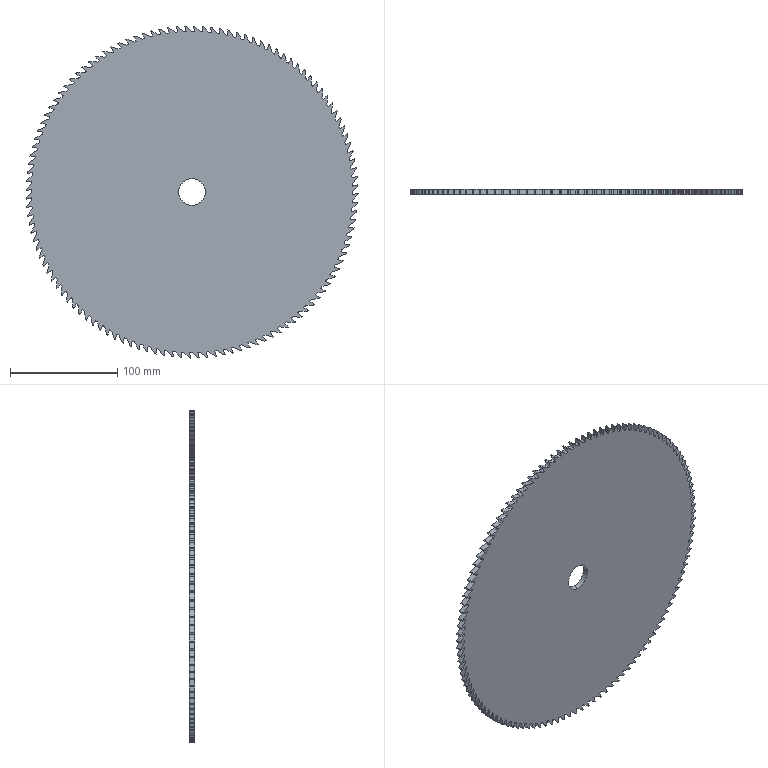Part | SolidWorks | features Extrusion 1, ICE 1 | 1 solid | 484 faces | box 309.988 x 5 x 309.988 mm | volume 361074 mm3 | cylinder 242 | plane 242 | commonest cylinder face diameters 300 x120 310 x120 25 x2